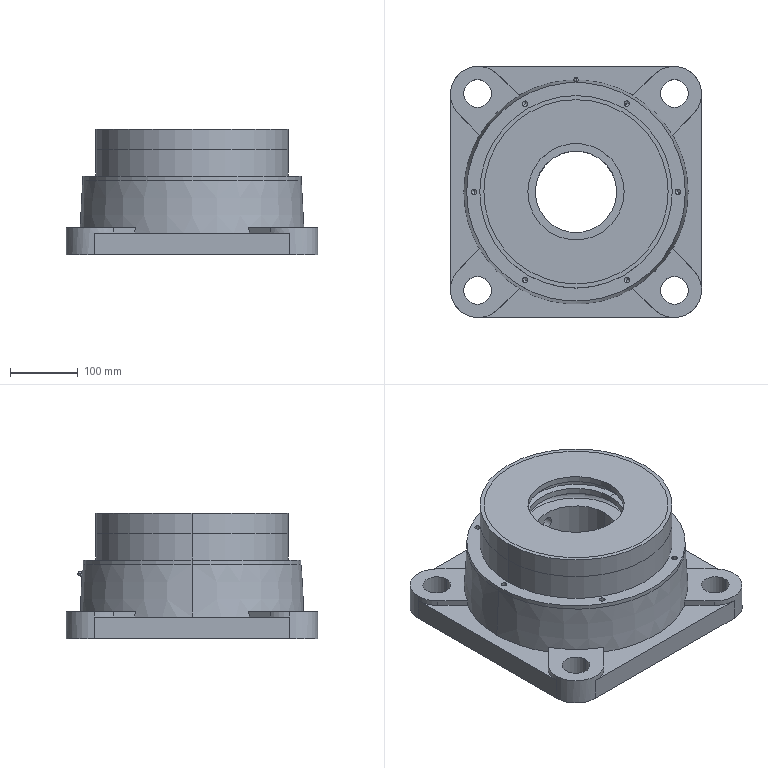Part | SolidWorks | features Revolution 5, RevCut 3, Boss 2, CirPattern 2, ICE 2, Cut 1, Extrusion 1, HoleWzd 1, RevolutionThin 1 | 2 solids | 164 faces | box 370 x 370 x 185 mm | volume 8271965 mm3 | cylinder 84 | plane 46 | cone 18 | sphere 10 | torus 6 | commonest cylinder face diameters 6 x14 8 x12 82 x12 41 x8 283.4 x8 160.6 x6